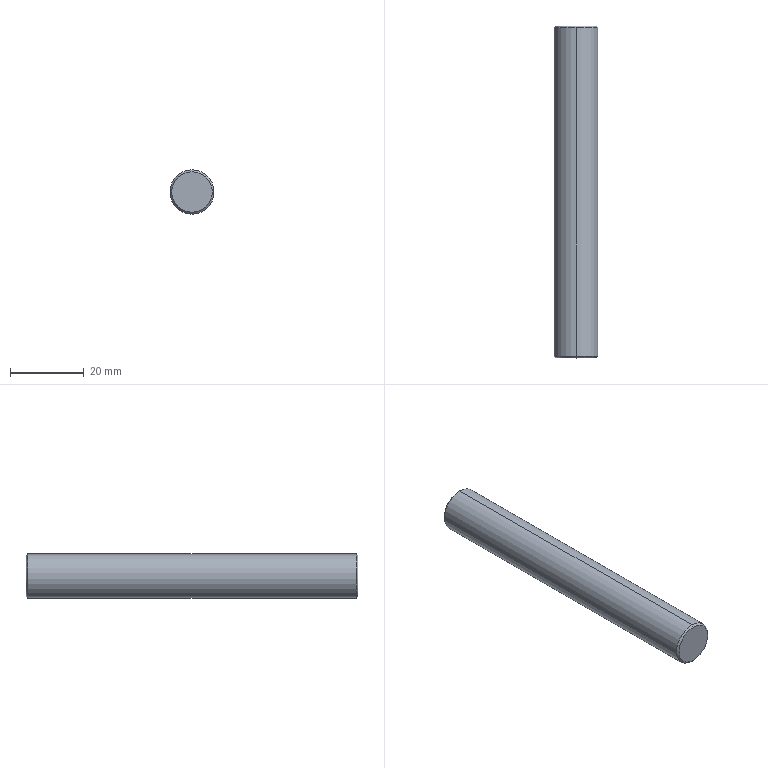Part | STEP file | ND25021-01-JDKM-15-GJ | 1 solid | 8 faces | box 12 x 90 x 12 mm | volume 10170 mm3 | cone 4 | cylinder 2 | plane 2 | commonest cylinder face diameters 12 x2
STEP:
#1=CARTESIAN_POINT('',(0.,0.,0.));
#2=DIRECTION('',(0.,0.,1.));
#3=DIRECTION('',(1.,0.,0.));
#4=AXIS2_PLACEMENT_3D('',#1,#2,#3);
#5=CARTESIAN_POINT('',(0.,-45.,-5.5));
#6=VERTEX_POINT('',#5);
#7=CARTESIAN_POINT('',(0.,-45.,5.5));
#8=VERTEX_POINT('',#7);
#9=CARTESIAN_POINT('',(0.,-45.,0.));
#10=DIRECTION('',(0.,-1.,0.));
#11=DIRECTION('',(0.,0.,1.));
#12=AXIS2_PLACEMENT_3D('',#9,#10,#11);
#13=CIRCLE('',#12,5.5);
#14=CARTESIAN_POINT('',(0.,-44.5,0.));
#15=DIRECTION('',(0.,1.,0.));
#16=DIRECTION('',(0.,0.,1.));
#17=AXIS2_PLACEMENT_3D('',#14,#15,#16);
#18=CONICAL_SURFACE('',#17,6.,0.7854);
#19=CARTESIAN_POINT('',(6.283,-0.5));
#20=DIRECTION('',(-1.,0.));
#21=VECTOR('',#20,1.);
#22=LINE('',#19,#21);
#23=(GEOMETRIC_REPRESENTATION_CONTEXT(2)PARAMETRIC_REPRESENTATION_CONTEXT()REPRESENTATION_CONTEXT('',''));
#24=DEFINITIONAL_REPRESENTATION('',(#22),#23);
#25=PCURVE('',#18,#24);
#26=CARTESIAN_POINT('',(0.,-45.,0.));
#27=DIRECTION('',(0.,1.,0.));
#28=DIRECTION('',(0.,0.,1.));
#29=AXIS2_PLACEMENT_3D('',#26,#27,#28);
#30=PLANE('',#29);
#31=CARTESIAN_POINT('',(5.5,0.));
#32=CARTESIAN_POINT('',(5.5,-9.526));
#33=CARTESIAN_POINT('',(-2.75,-4.763));
#34=CARTESIAN_POINT('',(-11.,0.));
#35=CARTESIAN_POINT('',(-2.75,4.763));
#36=CARTESIAN_POINT('',(5.5,9.526));
#37=CARTESIAN_POINT('',(5.5,0.));
#38=(BOUNDED_CURVE()B_SPLINE_CURVE(2,(#31,#32,#33,#34,#35,#36,#37),.UNSPECIFIED.,.T.,.F.)B_SPLINE_CURVE_WITH_KNOTS((1,2,2,2,2,1),(-2.094,0.,2.094,4.189,6.283,8.378),.UNSPECIFIED.)CURVE()GEOMETRIC_REPRESENTATION_ITEM()RATIONAL_B_SPLINE_CURVE((1.,0.5,1.,0.5,1.,0.5,1.))REPRESENTATION_ITEM(''));
#39=(GEOMETRIC_REPRESENTATION_CONTEXT(2)PARAMETRIC_REPRESENTATION_CONTEXT()REPRESENTATION_CONTEXT('',''));
#40=DEFINITIONAL_REPRESENTATION('',(#38),#39);
#41=PCURVE('',#30,#40);
#42=SURFACE_CURVE('',#13,(#25,#41),.PCURVE_S1.);
#43=EDGE_CURVE('',#6,#8,#42,.T.);
#44=ORIENTED_EDGE('',*,*,#43,.F.);
#45=CARTESIAN_POINT('',(0.,-44.5,-6.));
#46=VERTEX_POINT('',#45);
#47=CARTESIAN_POINT('',(0.,-44.5,-6.));
#48=DIRECTION('',(0.,0.7071,-0.7071));
#49=VECTOR('',#48,1.);
#50=LINE('',#47,#49);
#51=CARTESIAN_POINT('',(3.142,0.));
#52=DIRECTION('',(0.,1.));
#53=VECTOR('',#52,1.);
#54=LINE('',#51,#53);
#55=(GEOMETRIC_REPRESENTATION_CONTEXT(2)PARAMETRIC_REPRESENTATION_CONTEXT()REPRESENTATION_CONTEXT('',''));
#56=DEFINITIONAL_REPRESENTATION('',(#54),#55);
#57=PCURVE('',#18,#56);
#58=CARTESIAN_POINT('',(0.,-44.5,0.));
#59=DIRECTION('',(0.,1.,0.));
#60=DIRECTION('',(0.,0.,1.));
#61=AXIS2_PLACEMENT_3D('',#58,#59,#60);
#62=CONICAL_SURFACE('',#61,6.,0.7854);
#63=CARTESIAN_POINT('',(3.142,0.));
#64=DIRECTION('',(0.,1.));
#65=VECTOR('',#64,1.);
#66=LINE('',#63,#65);
#67=(GEOMETRIC_REPRESENTATION_CONTEXT(2)PARAMETRIC_REPRESENTATION_CONTEXT()REPRESENTATION_CONTEXT('',''));
#68=DEFINITIONAL_REPRESENTATION('',(#66),#67);
#69=PCURVE('',#62,#68);
#70=SURFACE_CURVE('',#50,(#57,#69),.PCURVE_S1.);
#71=EDGE_CURVE('',#6,#46,#70,.T.);
#72=ORIENTED_EDGE('',*,*,#71,.T.);
#73=CARTESIAN_POINT('',(0.,-44.5,6.));
#74=VERTEX_POINT('',#73);
#75=CARTESIAN_POINT('',(0.,-44.5,0.));
#76=DIRECTION('',(0.,1.,0.));
#77=DIRECTION('',(0.,0.,1.));
#78=AXIS2_PLACEMENT_3D('',#75,#76,#77);
#79=CIRCLE('',#78,6.);
#80=CARTESIAN_POINT('',(0.,0.));
#81=DIRECTION('',(1.,0.));
#82=VECTOR('',#81,1.);
#83=LINE('',#80,#82);
#84=(GEOMETRIC_REPRESENTATION_CONTEXT(2)PARAMETRIC_REPRESENTATION_CONTEXT()REPRESENTATION_CONTEXT('',''));
#85=DEFINITIONAL_REPRESENTATION('',(#83),#84);
#86=PCURVE('',#18,#85);
#87=CARTESIAN_POINT('',(0.,45.,0.));
#88=DIRECTION('',(0.,-1.,0.));
#89=DIRECTION('',(0.,0.,-1.));
#90=AXIS2_PLACEMENT_3D('',#87,#88,#89);
#91=CYLINDRICAL_SURFACE('',#90,6.);
#92=CARTESIAN_POINT('',(3.142,89.5));
#93=DIRECTION('',(-1.,0.));
#94=VECTOR('',#93,1.);
#95=LINE('',#92,#94);
#96=(GEOMETRIC_REPRESENTATION_CONTEXT(2)PARAMETRIC_REPRESENTATION_CONTEXT()REPRESENTATION_CONTEXT('',''));
#97=DEFINITIONAL_REPRESENTATION('',(#95),#96);
#98=PCURVE('',#91,#97);
#99=SURFACE_CURVE('',#79,(#86,#98),.PCURVE_S1.);
#100=EDGE_CURVE('',#74,#46,#99,.T.);
#101=ORIENTED_EDGE('',*,*,#100,.F.);
#102=CARTESIAN_POINT('',(0.,-44.5,6.));
#103=DIRECTION('',(0.,0.7071,0.7071));
#104=VECTOR('',#103,1.);
#105=LINE('',#102,#104);
#106=CARTESIAN_POINT('',(0.,0.));
#107=DIRECTION('',(0.,1.));
#108=VECTOR('',#107,1.);
#109=LINE('',#106,#108);
#110=(GEOMETRIC_REPRESENTATION_CONTEXT(2)PARAMETRIC_REPRESENTATION_CONTEXT()REPRESENTATION_CONTEXT('',''));
#111=DEFINITIONAL_REPRESENTATION('',(#109),#110);
#112=PCURVE('',#18,#111);
#113=CARTESIAN_POINT('',(6.283,0.));
#114=DIRECTION('',(0.,1.));
#115=VECTOR('',#114,1.);
#116=LINE('',#113,#115);
#117=(GEOMETRIC_REPRESENTATION_CONTEXT(2)PARAMETRIC_REPRESENTATION_CONTEXT()REPRESENTATION_CONTEXT('',''));
#118=DEFINITIONAL_REPRESENTATION('',(#116),#117);
#119=PCURVE('',#62,#118);
#120=SURFACE_CURVE('',#105,(#112,#119),.PCURVE_S1.);
#121=EDGE_CURVE('',#8,#74,#120,.T.);
#122=ORIENTED_EDGE('',*,*,#121,.F.);
#123=EDGE_LOOP('',(#44,#72,#101,#122));
#124=FACE_BOUND('',#123,.T.);
#125=ADVANCED_FACE('',(#124),#18,.T.);
#126=CARTESIAN_POINT('',(0.,45.,5.5));
#127=VERTEX_POINT('',#126);
#128=CARTESIAN_POINT('',(0.,45.,-5.5));
#129=VERTEX_POINT('',#128);
#130=CARTESIAN_POINT('',(0.,45.,0.));
#131=DIRECTION('',(0.,1.,0.));
#132=DIRECTION('',(0.,0.,1.));
#133=AXIS2_PLACEMENT_3D('',#130,#131,#132);
#134=CIRCLE('',#133,5.5);
#135=CARTESIAN_POINT('',(0.,45.,0.));
#136=DIRECTION('',(0.,-1.,0.));
#137=DIRECTION('',(0.,0.,-1.));
#138=AXIS2_PLACEMENT_3D('',#135,#136,#137);
#139=CONICAL_SURFACE('',#138,5.5,0.7854);
#140=CARTESIAN_POINT('',(3.142,0.));
#141=DIRECTION('',(-1.,0.));
#142=VECTOR('',#141,1.);
#143=LINE('',#140,#142);
#144=(GEOMETRIC_REPRESENTATION_CONTEXT(2)PARAMETRIC_REPRESENTATION_CONTEXT()REPRESENTATION_CONTEXT('',''));
#145=DEFINITIONAL_REPRESENTATION('',(#143),#144);
#146=PCURVE('',#139,#145);
#147=CARTESIAN_POINT('',(0.,45.,0.));
#148=DIRECTION('',(0.,1.,0.));
#149=DIRECTION('',(0.,0.,1.));
#150=AXIS2_PLACEMENT_3D('',#147,#148,#149);
#151=PLANE('',#150);
#152=CARTESIAN_POINT('',(0.,0.));
#153=DIRECTION('',(1.,0.));
#154=AXIS2_PLACEMENT_2D('',#152,#153);
#155=CIRCLE('',#154,5.5);
#156=(GEOMETRIC_REPRESENTATION_CONTEXT(2)PARAMETRIC_REPRESENTATION_CONTEXT()REPRESENTATION_CONTEXT('',''));
#157=DEFINITIONAL_REPRESENTATION('',(#155),#156);
#158=PCURVE('',#151,#157);
#159=SURFACE_CURVE('',#134,(#146,#158),.PCURVE_S1.);
#160=EDGE_CURVE('',#127,#129,#159,.T.);
#161=ORIENTED_EDGE('',*,*,#160,.F.);
#162=CARTESIAN_POINT('',(0.,44.5,6.));
#163=VERTEX_POINT('',#162);
#164=CARTESIAN_POINT('',(0.,45.,5.5));
#165=DIRECTION('',(0.,-0.7071,0.7071));
#166=VECTOR('',#165,1.);
#167=LINE('',#164,#166);
#168=CARTESIAN_POINT('',(3.142,0.));
#169=DIRECTION('',(0.,1.));
#170=VECTOR('',#169,1.);
#171=LINE('',#168,#170);
#172=(GEOMETRIC_REPRESENTATION_CONTEXT(2)PARAMETRIC_REPRESENTATION_CONTEXT()REPRESENTATION_CONTEXT('',''));
#173=DEFINITIONAL_REPRESENTATION('',(#171),#172);
#174=PCURVE('',#139,#173);
#175=CARTESIAN_POINT('',(0.,45.,0.));
#176=DIRECTION('',(0.,-1.,0.));
#177=DIRECTION('',(0.,0.,-1.));
#178=AXIS2_PLACEMENT_3D('',#175,#176,#177);
#179=CONICAL_SURFACE('',#178,5.5,0.7854);
#180=CARTESIAN_POINT('',(3.142,0.));
#181=DIRECTION('',(0.,1.));
#182=VECTOR('',#181,1.);
#183=LINE('',#180,#182);
#184=(GEOMETRIC_REPRESENTATION_CONTEXT(2)PARAMETRIC_REPRESENTATION_CONTEXT()REPRESENTATION_CONTEXT('',''));
#185=DEFINITIONAL_REPRESENTATION('',(#183),#184);
#186=PCURVE('',#179,#185);
#187=SURFACE_CURVE('',#167,(#174,#186),.PCURVE_S1.);
#188=EDGE_CURVE('',#127,#163,#187,.T.);
#189=ORIENTED_EDGE('',*,*,#188,.T.);
#190=CARTESIAN_POINT('',(0.,44.5,-6.));
#191=VERTEX_POINT('',#190);
#192=CARTESIAN_POINT('',(0.,44.5,0.));
#193=DIRECTION('',(0.,-1.,0.));
#194=DIRECTION('',(0.,0.,1.));
#195=AXIS2_PLACEMENT_3D('',#192,#193,#194);
#196=CIRCLE('',#195,6.);
#197=CARTESIAN_POINT('',(-3.142,0.5));
#198=DIRECTION('',(1.,0.));
#199=VECTOR('',#198,1.);
#200=LINE('',#197,#199);
#201=(GEOMETRIC_REPRESENTATION_CONTEXT(2)PARAMETRIC_REPRESENTATION_CONTEXT()REPRESENTATION_CONTEXT('',''));
#202=DEFINITIONAL_REPRESENTATION('',(#200),#201);
#203=PCURVE('',#139,#202);
#204=CARTESIAN_POINT('',(-3.142,0.5));
#205=DIRECTION('',(1.,0.));
#206=VECTOR('',#205,1.);
#207=LINE('',#204,#206);
#208=(GEOMETRIC_REPRESENTATION_CONTEXT(2)PARAMETRIC_REPRESENTATION_CONTEXT()REPRESENTATION_CONTEXT('',''));
#209=DEFINITIONAL_REPRESENTATION('',(#207),#208);
#210=PCURVE('',#91,#209);
#211=SURFACE_CURVE('',#196,(#203,#210),.PCURVE_S1.);
#212=EDGE_CURVE('',#191,#163,#211,.T.);
#213=ORIENTED_EDGE('',*,*,#212,.F.);
#214=CARTESIAN_POINT('',(0.,45.,-5.5));
#215=DIRECTION('',(0.,-0.7071,-0.7071));
#216=VECTOR('',#215,1.);
#217=LINE('',#214,#216);
#218=CARTESIAN_POINT('',(0.,0.));
#219=DIRECTION('',(0.,1.));
#220=VECTOR('',#219,1.);
#221=LINE('',#218,#220);
#222=(GEOMETRIC_REPRESENTATION_CONTEXT(2)PARAMETRIC_REPRESENTATION_CONTEXT()REPRESENTATION_CONTEXT('',''));
#223=DEFINITIONAL_REPRESENTATION('',(#221),#222);
#224=PCURVE('',#139,#223);
#225=CARTESIAN_POINT('',(6.283,0.));
#226=DIRECTION('',(0.,1.));
#227=VECTOR('',#226,1.);
#228=LINE('',#225,#227);
#229=(GEOMETRIC_REPRESENTATION_CONTEXT(2)PARAMETRIC_REPRESENTATION_CONTEXT()REPRESENTATION_CONTEXT('',''));
#230=DEFINITIONAL_REPRESENTATION('',(#228),#229);
#231=PCURVE('',#179,#230);
#232=SURFACE_CURVE('',#217,(#224,#231),.PCURVE_S1.);
#233=EDGE_CURVE('',#129,#191,#232,.T.);
#234=ORIENTED_EDGE('',*,*,#233,.F.);
#235=EDGE_LOOP('',(#161,#189,#213,#234));
#236=FACE_BOUND('',#235,.T.);
#237=ADVANCED_FACE('',(#236),#139,.T.);
#238=ORIENTED_EDGE('',*,*,#212,.T.);
#239=CARTESIAN_POINT('',(0.,45.,6.));
#240=DIRECTION('',(0.,-1.,0.));
#241=VECTOR('',#240,1.);
#242=LINE('',#239,#241);
#243=CARTESIAN_POINT('',(3.142,0.));
#244=DIRECTION('',(0.,1.));
#245=VECTOR('',#244,1.);
#246=LINE('',#243,#245);
#247=(GEOMETRIC_REPRESENTATION_CONTEXT(2)PARAMETRIC_REPRESENTATION_CONTEXT()REPRESENTATION_CONTEXT('',''));
#248=DEFINITIONAL_REPRESENTATION('',(#246),#247);
#249=PCURVE('',#91,#248);
#250=CARTESIAN_POINT('',(0.,45.,0.));
#251=DIRECTION('',(0.,-1.,0.));
#252=DIRECTION('',(0.,0.,-1.));
#253=AXIS2_PLACEMENT_3D('',#250,#251,#252);
#254=CYLINDRICAL_SURFACE('',#253,6.);
#255=CARTESIAN_POINT('',(3.142,0.));
#256=DIRECTION('',(0.,1.));
#257=VECTOR('',#256,1.);
#258=LINE('',#255,#257);
#259=(GEOMETRIC_REPRESENTATION_CONTEXT(2)PARAMETRIC_REPRESENTATION_CONTEXT()REPRESENTATION_CONTEXT('',''));
#260=DEFINITIONAL_REPRESENTATION('',(#258),#259);
#261=PCURVE('',#254,#260);
#262=SURFACE_CURVE('',#242,(#249,#261),.PCURVE_S1.);
#263=EDGE_CURVE('',#163,#74,#262,.T.);
#264=ORIENTED_EDGE('',*,*,#263,.T.);
#265=ORIENTED_EDGE('',*,*,#100,.T.);
#266=CARTESIAN_POINT('',(0.,45.,-6.));
#267=DIRECTION('',(0.,-1.,0.));
#268=VECTOR('',#267,1.);
#269=LINE('',#266,#268);
#270=CARTESIAN_POINT('',(0.,0.));
#271=DIRECTION('',(0.,1.));
#272=VECTOR('',#271,1.);
#273=LINE('',#270,#272);
#274=(GEOMETRIC_REPRESENTATION_CONTEXT(2)PARAMETRIC_REPRESENTATION_CONTEXT()REPRESENTATION_CONTEXT('',''));
#275=DEFINITIONAL_REPRESENTATION('',(#273),#274);
#276=PCURVE('',#91,#275);
#277=CARTESIAN_POINT('',(6.283,0.));
#278=DIRECTION('',(0.,1.));
#279=VECTOR('',#278,1.);
#280=LINE('',#277,#279);
#281=(GEOMETRIC_REPRESENTATION_CONTEXT(2)PARAMETRIC_REPRESENTATION_CONTEXT()REPRESENTATION_CONTEXT('',''));
#282=DEFINITIONAL_REPRESENTATION('',(#280),#281);
#283=PCURVE('',#254,#282);
#284=SURFACE_CURVE('',#269,(#276,#283),.PCURVE_S1.);
#285=EDGE_CURVE('',#191,#46,#284,.T.);
#286=ORIENTED_EDGE('',*,*,#285,.F.);
#287=EDGE_LOOP('',(#238,#264,#265,#286));
#288=FACE_BOUND('',#287,.T.);
#289=ADVANCED_FACE('',(#288),#91,.T.);
#290=ORIENTED_EDGE('',*,*,#263,.F.);
#291=CARTESIAN_POINT('',(0.,44.5,0.));
#292=DIRECTION('',(0.,-1.,0.));
#293=DIRECTION('',(0.,0.,1.));
#294=AXIS2_PLACEMENT_3D('',#291,#292,#293);
#295=CIRCLE('',#294,6.);
#296=CARTESIAN_POINT('',(3.142,0.5));
#297=DIRECTION('',(1.,0.));
#298=VECTOR('',#297,1.);
#299=LINE('',#296,#298);
#300=(GEOMETRIC_REPRESENTATION_CONTEXT(2)PARAMETRIC_REPRESENTATION_CONTEXT()REPRESENTATION_CONTEXT('',''));
#301=DEFINITIONAL_REPRESENTATION('',(#299),#300);
#302=PCURVE('',#254,#301);
#303=CARTESIAN_POINT('',(3.142,0.5));
#304=DIRECTION('',(1.,0.));
#305=VECTOR('',#304,1.);
#306=LINE('',#303,#305);
#307=(GEOMETRIC_REPRESENTATION_CONTEXT(2)PARAMETRIC_REPRESENTATION_CONTEXT()REPRESENTATION_CONTEXT('',''));
#308=DEFINITIONAL_REPRESENTATION('',(#306),#307);
#309=PCURVE('',#179,#308);
#310=SURFACE_CURVE('',#295,(#302,#309),.PCURVE_S1.);
#311=EDGE_CURVE('',#163,#191,#310,.T.);
#312=ORIENTED_EDGE('',*,*,#311,.T.);
#313=ORIENTED_EDGE('',*,*,#285,.T.);
#314=CARTESIAN_POINT('',(0.,-44.5,0.));
#315=DIRECTION('',(0.,1.,0.));
#316=DIRECTION('',(0.,0.,1.));
#317=AXIS2_PLACEMENT_3D('',#314,#315,#316);
#318=CIRCLE('',#317,6.);
#319=CARTESIAN_POINT('',(9.425,89.5));
#320=DIRECTION('',(-1.,0.));
#321=VECTOR('',#320,1.);
#322=LINE('',#319,#321);
#323=(GEOMETRIC_REPRESENTATION_CONTEXT(2)PARAMETRIC_REPRESENTATION_CONTEXT()REPRESENTATION_CONTEXT('',''));
#324=DEFINITIONAL_REPRESENTATION('',(#322),#323);
#325=PCURVE('',#254,#324);
#326=CARTESIAN_POINT('',(0.,0.));
#327=DIRECTION('',(1.,0.));
#328=VECTOR('',#327,1.);
#329=LINE('',#326,#328);
#330=(GEOMETRIC_REPRESENTATION_CONTEXT(2)PARAMETRIC_REPRESENTATION_CONTEXT()REPRESENTATION_CONTEXT('',''));
#331=DEFINITIONAL_REPRESENTATION('',(#329),#330);
#332=PCURVE('',#62,#331);
#333=SURFACE_CURVE('',#318,(#325,#332),.PCURVE_S1.);
#334=EDGE_CURVE('',#46,#74,#333,.T.);
#335=ORIENTED_EDGE('',*,*,#334,.T.);
#336=EDGE_LOOP('',(#290,#312,#313,#335));
#337=FACE_BOUND('',#336,.T.);
#338=ADVANCED_FACE('',(#337),#254,.T.);
#339=CARTESIAN_POINT('',(0.,45.,0.));
#340=DIRECTION('',(0.,1.,0.));
#341=DIRECTION('',(0.,0.,1.));
#342=AXIS2_PLACEMENT_3D('',#339,#340,#341);
#343=CIRCLE('',#342,5.5);
#344=CARTESIAN_POINT('',(0.,0.));
#345=DIRECTION('',(1.,0.));
#346=AXIS2_PLACEMENT_2D('',#344,#345);
#347=CIRCLE('',#346,5.5);
#348=(GEOMETRIC_REPRESENTATION_CONTEXT(2)PARAMETRIC_REPRESENTATION_CONTEXT()REPRESENTATION_CONTEXT('',''));
#349=DEFINITIONAL_REPRESENTATION('',(#347),#348);
#350=PCURVE('',#151,#349);
#351=CARTESIAN_POINT('',(9.425,0.));
#352=DIRECTION('',(-1.,0.));
#353=VECTOR('',#352,1.);
#354=LINE('',#351,#353);
#355=(GEOMETRIC_REPRESENTATION_CONTEXT(2)PARAMETRIC_REPRESENTATION_CONTEXT()REPRESENTATION_CONTEXT('',''));
#356=DEFINITIONAL_REPRESENTATION('',(#354),#355);
#357=PCURVE('',#179,#356);
#358=SURFACE_CURVE('',#343,(#350,#357),.PCURVE_S1.);
#359=EDGE_CURVE('',#129,#127,#358,.T.);
#360=ORIENTED_EDGE('',*,*,#359,.T.);
#361=ORIENTED_EDGE('',*,*,#160,.T.);
#362=EDGE_LOOP('',(#360,#361));
#363=FACE_BOUND('',#362,.T.);
#364=ADVANCED_FACE('',(#363),#151,.T.);
#365=CARTESIAN_POINT('',(0.,-45.,0.));
#366=DIRECTION('',(0.,-1.,0.));
#367=DIRECTION('',(0.,0.,1.));
#368=AXIS2_PLACEMENT_3D('',#365,#366,#367);
#369=CIRCLE('',#368,5.5);
#370=CARTESIAN_POINT('',(5.5,0.));
#371=CARTESIAN_POINT('',(5.5,-9.526));
#372=CARTESIAN_POINT('',(-2.75,-4.763));
#373=CARTESIAN_POINT('',(-11.,0.));
#374=CARTESIAN_POINT('',(-2.75,4.763));
#375=CARTESIAN_POINT('',(5.5,9.526));
#376=CARTESIAN_POINT('',(5.5,0.));
#377=(BOUNDED_CURVE()B_SPLINE_CURVE(2,(#370,#371,#372,#373,#374,#375,#376),.UNSPECIFIED.,.T.,.F.)B_SPLINE_CURVE_WITH_KNOTS((1,2,2,2,2,1),(-2.094,0.,2.094,4.189,6.283,8.378),.UNSPECIFIED.)CURVE()GEOMETRIC_REPRESENTATION_ITEM()RATIONAL_B_SPLINE_CURVE((1.,0.5,1.,0.5,1.,0.5,1.))REPRESENTATION_ITEM(''));
#378=(GEOMETRIC_REPRESENTATION_CONTEXT(2)PARAMETRIC_REPRESENTATION_CONTEXT()REPRESENTATION_CONTEXT('',''));
#379=DEFINITIONAL_REPRESENTATION('',(#377),#378);
#380=PCURVE('',#30,#379);
#381=CARTESIAN_POINT('',(6.283,-0.5));
#382=DIRECTION('',(-1.,0.));
#383=VECTOR('',#382,1.);
#384=LINE('',#381,#383);
#385=(GEOMETRIC_REPRESENTATION_CONTEXT(2)PARAMETRIC_REPRESENTATION_CONTEXT()REPRESENTATION_CONTEXT('',''));
#386=DEFINITIONAL_REPRESENTATION('',(#384),#385);
#387=PCURVE('',#62,#386);
#388=SURFACE_CURVE('',#369,(#380,#387),.PCURVE_S1.);
#389=EDGE_CURVE('',#8,#6,#388,.T.);
#390=ORIENTED_EDGE('',*,*,#389,.T.);
#391=ORIENTED_EDGE('',*,*,#43,.T.);
#392=EDGE_LOOP('',(#390,#391));
#393=FACE_BOUND('',#392,.T.);
#394=ADVANCED_FACE('',(#393),#30,.F.);
#395=ORIENTED_EDGE('',*,*,#188,.F.);
#396=ORIENTED_EDGE('',*,*,#359,.F.);
#397=ORIENTED_EDGE('',*,*,#233,.T.);
#398=ORIENTED_EDGE('',*,*,#311,.F.);
#399=EDGE_LOOP('',(#395,#396,#397,#398));
#400=FACE_BOUND('',#399,.T.);
#401=ADVANCED_FACE('',(#400),#179,.T.);
#402=ORIENTED_EDGE('',*,*,#71,.F.);
#403=ORIENTED_EDGE('',*,*,#389,.F.);
#404=ORIENTED_EDGE('',*,*,#121,.T.);
#405=ORIENTED_EDGE('',*,*,#334,.F.);
#406=EDGE_LOOP('',(#402,#403,#404,#405));
#407=FACE_BOUND('',#406,.T.);
#408=ADVANCED_FACE('',(#407),#62,.T.);
#409=CLOSED_SHELL('',(#125,#237,#289,#338,#364,#394,#401,#408));
#410=MANIFOLD_SOLID_BREP('',#409);
#411=(LENGTH_UNIT()NAMED_UNIT(*)SI_UNIT(.MILLI.,.METRE.));
#412=UNCERTAINTY_MEASURE_WITH_UNIT(LENGTH_MEASURE(0.0000001),#411,'','');
#413=(NAMED_UNIT(*)PLANE_ANGLE_UNIT()SI_UNIT($,.RADIAN.));
#414=(NAMED_UNIT(*)SI_UNIT($,.STERADIAN.)SOLID_ANGLE_UNIT());
#415=(GEOMETRIC_REPRESENTATION_CONTEXT(3)GLOBAL_UNCERTAINTY_ASSIGNED_CONTEXT((#412))GLOBAL_UNIT_ASSIGNED_CONTEXT((#411,#413,#414))REPRESENTATION_CONTEXT('',''));
#416=ADVANCED_BREP_SHAPE_REPRESENTATION('',(#4,#410),#415);